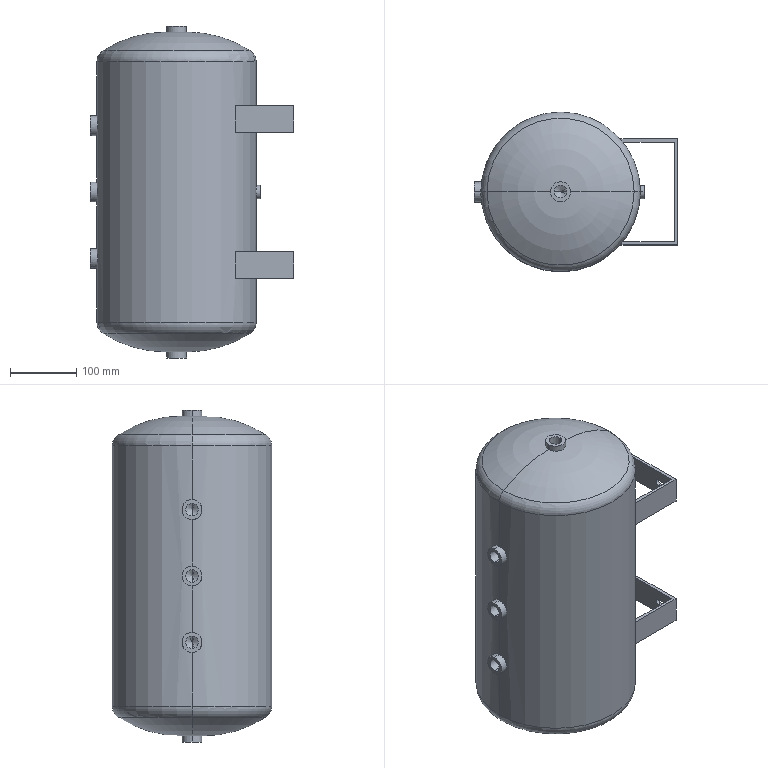Part | SolidWorks | features ICE 5, HoleWzd 4, MirrorPattern 3, RefAxis 2, Extrusion 1, Revolution 1 | 1 solid | 84 faces | box 306.443 x 240 x 500 mm | volume 20512353 mm3 | cylinder 34 | plane 30 | cone 12 | torus 8 | commonest cylinder face diameters 19 x10 30 x10 9 x8 11.8 x2 20 x2 240 x2